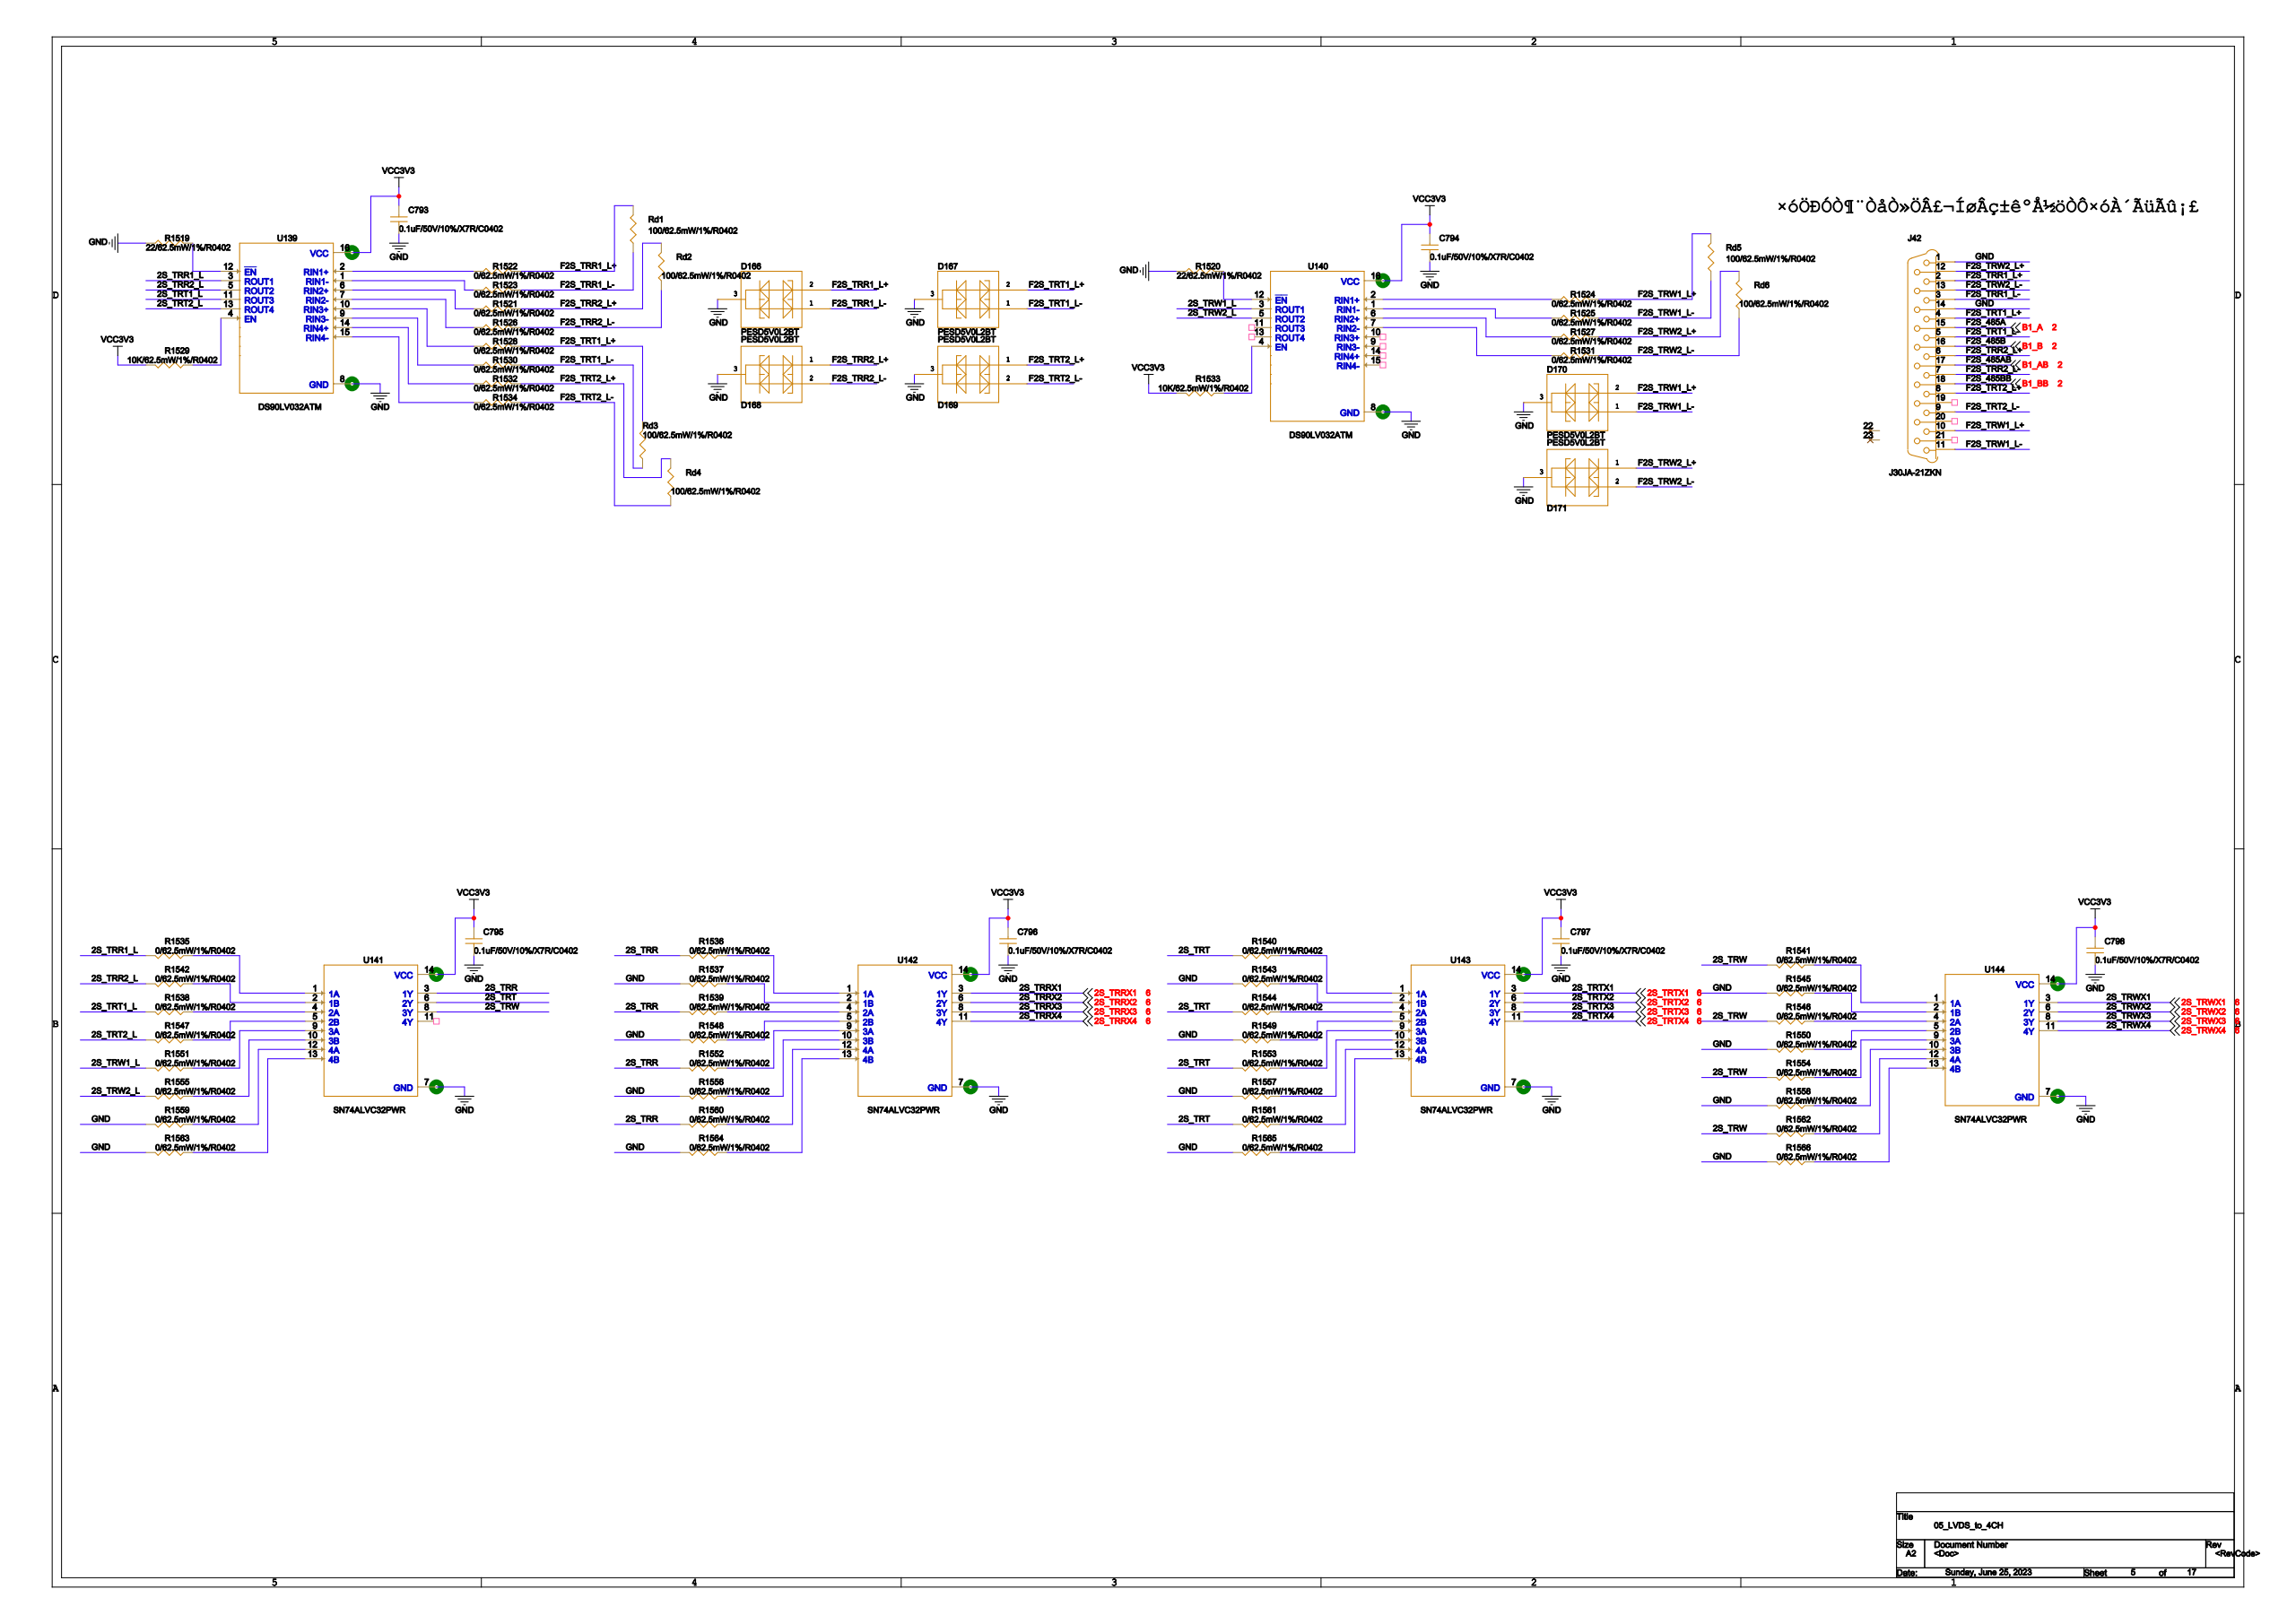Circuit board | Cadence Allegro | 1997 parts | 1536 nets | one sheet of the schematic
Parts on this sheet (reference | value | footprint):
C793 | 0.1uF/50V/10%/X7R/C0402 | 0402
C794 | 0.1uF/50V/10%/X7R/C0402 | 0402
C795 | 0.1uF/50V/10%/X7R/C0402 | 0402
C796 | 0.1uF/50V/10%/X7R/C0402 | 0402
C797 | 0.1uF/50V/10%/X7R/C0402 | 0402
C798 | 0.1uF/50V/10%/X7R/C0402 | 0402
D166 | PESD5V0L2BT | SOT23
D167 | PESD5V0L2BT | SOT23
D168 | PESD5V0L2BT | SOT23
D169 | PESD5V0L2BT | SOT23
D170 | PESD5V0L2BT | SOT23
D171 | PESD5V0L2BT | SOT23
J42 | J30JA-21ZKN | J30JA-21ZKN
R1519 | 22/62.5mW/1%/R0402 | 0402
R1520 | 22/62.5mW/1%/R0402 | 0402
R1521 | 0/62.5mW/1%/R0402 | 0402
R1522 | 0/62.5mW/1%/R0402 | 0402
R1523 | 0/62.5mW/1%/R0402 | 0402
R1524 | 0/62.5mW/1%/R0402 | 0402
R1525 | 0/62.5mW/1%/R0402 | 0402
R1526 | 0/62.5mW/1%/R0402 | 0402
R1527 | 0/62.5mW/1%/R0402 | 0402
R1528 | 0/62.5mW/1%/R0402 | 0402
R1529 | 10K/62.5mW/1%/R0402 | 0402
R1530 | 0/62.5mW/1%/R0402 | 0402
R1531 | 0/62.5mW/1%/R0402 | 0402
R1532 | 0/62.5mW/1%/R0402 | 0402
R1533 | 10K/62.5mW/1%/R0402 | 0402
R1534 | 0/62.5mW/1%/R0402 | 0402
R1535 | 0/62.5mW/1%/R0402 | 0402
R1536 | 0/62.5mW/1%/R0402 | 0402
R1537 | 0/62.5mW/1%/R0402 | 0402
R1538 | 0/62.5mW/1%/R0402 | 0402
R1539 | 0/62.5mW/1%/R0402 | 0402
R1540 | 0/62.5mW/1%/R0402 | 0402
R1541 | 0/62.5mW/1%/R0402 | 0402
R1542 | 0/62.5mW/1%/R0402 | 0402
R1543 | 0/62.5mW/1%/R0402 | 0402
R1544 | 0/62.5mW/1%/R0402 | 0402
R1545 | 0/62.5mW/1%/R0402 | 0402
R1546 | 0/62.5mW/1%/R0402 | 0402
R1547 | 0/62.5mW/1%/R0402 | 0402
R1548 | 0/62.5mW/1%/R0402 | 0402
R1549 | 0/62.5mW/1%/R0402 | 0402
R1550 | 0/62.5mW/1%/R0402 | 0402
R1551 | 0/62.5mW/1%/R0402 | 0402
R1552 | 0/62.5mW/1%/R0402 | 0402
R1553 | 0/62.5mW/1%/R0402 | 0402
R1554 | 0/62.5mW/1%/R0402 | 0402
R1555 | 0/62.5mW/1%/R0402 | 0402
R1556 | 0/62.5mW/1%/R0402 | 0402
R1557 | 0/62.5mW/1%/R0402 | 0402
R1558 | 0/62.5mW/1%/R0402 | 0402
R1559 | 0/62.5mW/1%/R0402 | 0402
R1560 | 0/62.5mW/1%/R0402 | 0402
R1561 | 0/62.5mW/1%/R0402 | 0402
R1562 | 0/62.5mW/1%/R0402 | 0402
R1563 | 0/62.5mW/1%/R0402 | 0402
R1564 | 0/62.5mW/1%/R0402 | 0402
R1565 | 0/62.5mW/1%/R0402 | 0402
R1566 | 0/62.5mW/1%/R0402 | 0402
U139 | DS90LV032ATM | SOIC127P600X175-16N
U140 | DS90LV032ATM | SOIC127P600X175-16N
U141 | SN74ALVC32PWR | SOP65P640X120-14N
U142 | SN74ALVC32PWR | SOP65P640X120-14N
U143 | SN74ALVC32PWR | SOP65P640X120-14N
U144 | SN74ALVC32PWR | SOP65P640X120-14N
Nets of these parts (net: part-pin ...):
3.3V: C793-1 C794-1 C795-1 C796-1 C797-1 C798-1 R1529-1 R1533-1 U139-16 U140-16 U141-14 U142-14 U143-14 U144-14
AGND: C793-2 C794-2 C795-2 C796-2 C797-2 C798-2 D166-3 D167-3 D168-3 D169-3 D170-3 D171-3 J42-1 J42-14 R1519-2 R1520-2 R1537-1 R1543-1 R1545-1 R1548-1 R1549-1 R1550-1 R1556-1 R1557-1 R1558-1 R1559-1 R1563-1 R1564-1 R1565-1 R1566-1 U139-8 U140-8 U141-7 U142-7 U143-7 U144-7
F2S_TRW1_L+: D170-2 J42-10 R1524-1
F2S_TRW1_L-: D170-1 J42-11 R1525-1
F2S_TRW2_L+: D171-1 J42-12 R1527-1
F2S_TRW2_L-: D171-2 J42-13 R1531-1
B1_A: J42-15
B1_B: J42-16
B1_AB: J42-17
B1_BB: J42-18
F2S_TRR1_L+: D166-2 J42-2 R1522-1
F2S_TRR1_L-: D166-1 J42-3 R1523-1
F2S_TRT1_L+: D167-2 J42-4 R1528-1
F2S_TRT1_L-: D167-1 J42-5 R1530-1
F2S_TRR2_L+: D168-1 J42-6 R1521-1
F2S_TRR2_L-: D168-2 J42-7 R1526-1
F2S_TRT2_L+: D169-1 J42-8 R1532-1
F2S_TRT2_L-: D169-2 J42-9 R1534-1
N23932818: R1521-2 U139-6
N23932828: R1522-2 U139-2
N23932816: R1523-2 U139-1
N23933318: R1524-2 U140-2
N23933306: R1525-2 U140-1
N23932814: R1526-2 U139-7
N23933308: R1527-2 U140-6
N23932880: R1528-2 U139-10
N23932860: R1530-2 U139-9
N23933304: R1531-2 U140-7
N23932862: R1532-2 U139-14
N23932858: R1534-2 U139-15
2S_TRR1_L: R1535-1 U139-3
N23947474: R1535-2 U141-1
2S_TRR: R1536-1 R1539-1 R1552-1 R1560-1 U141-3
N23951252: R1536-2 U142-1
N23951246: R1537-2 U142-2
2S_TRT1_L: R1538-1 U139-11
N23947464: R1538-2 U141-4
N23951241: R1539-2 U142-4
2S_TRT: R1540-1 R1544-1 R1553-1 R1561-1 U141-6
N23952028: R1540-2 U143-1
2S_TRW: R1541-1 R1546-1 R1554-1 R1562-1 U141-8
N23952637: R1541-2 U144-1
2S_TRR2_L: R1542-1 U139-5
N23947468: R1542-2 U141-2
N23952022: R1543-2 U143-2
N23952017: R1544-2 U143-4
N23952631: R1545-2 U144-2
N23952626: R1546-2 U144-4
2S_TRT2_L: R1547-1 U139-13
N23947458: R1547-2 U141-5
N23951235: R1548-2 U142-5
N23952011: R1549-2 U143-5
N23952620: R1550-2 U144-5
2S_TRW1_L: R1551-1 U140-3
N23947916: R1551-2 U141-9
N23951299: R1552-2 U142-9
N23952075: R1553-2 U143-9
N23952684: R1554-2 U144-9
2S_TRW2_L: R1555-1 U140-5
N23947925: R1555-2 U141-10
N23951313: R1556-2 U142-10
N23952089: R1557-2 U143-10
N23952698: R1558-2 U144-10
N23948082: R1559-2 U141-12
N23951333: R1560-2 U142-12
N23952098: R1561-2 U143-12
N23952707: R1562-2 U144-12
N23948113: R1563-2 U141-13
N23951346: R1564-2 U142-13
N23952119: R1565-2 U143-13
N23952728: R1566-2 U144-13
2S_TRRX1: U142-3
2S_TRTX1: U143-3
2S_TRWX1: U144-3
2S_TRRX2: U142-6
2S_TRTX2: U143-6
2S_TRWX2: U144-6
2S_TRRX3: U142-8
2S_TRTX3: U143-8
2S_TRWX3: U144-8
2S_TRRX4: U142-11
2S_TRTX4: U143-11
2S_TRWX4: U144-11
N23932768: R1529-2 U139-4
N23932772: R1519-1 U139-12
N23933268: R1533-2 U140-4
N23933272: R1520-1 U140-12